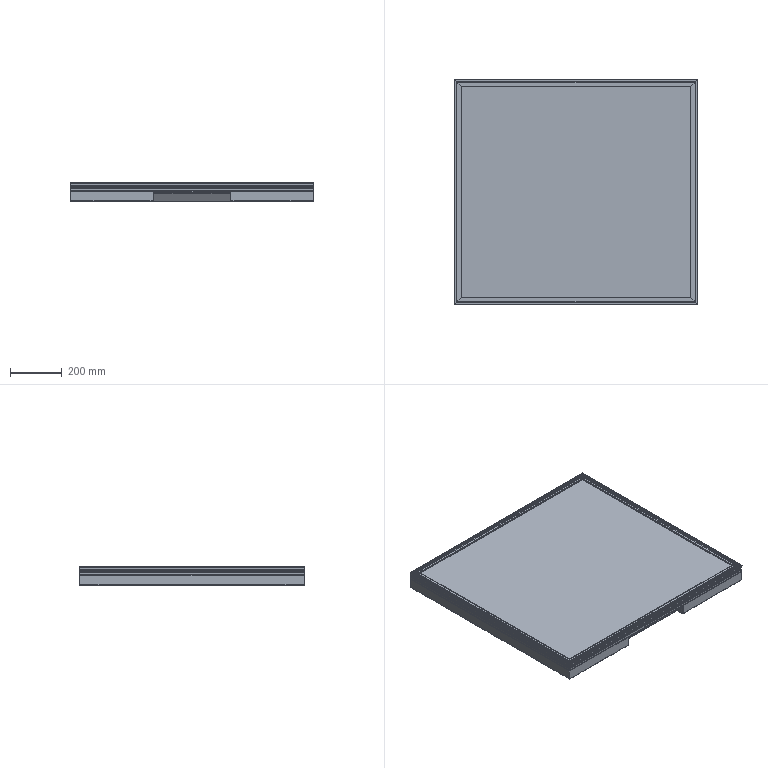Part | 9 solids | 878 faces | box 940 x 870 x 70 mm | volume 15170023 mm3 | plane 582 | cylinder 264 | spline 32 | commonest cylinder face diameters 7 x100 0.4 x67 2.4 x41 11 x32 2 x16 1 x8